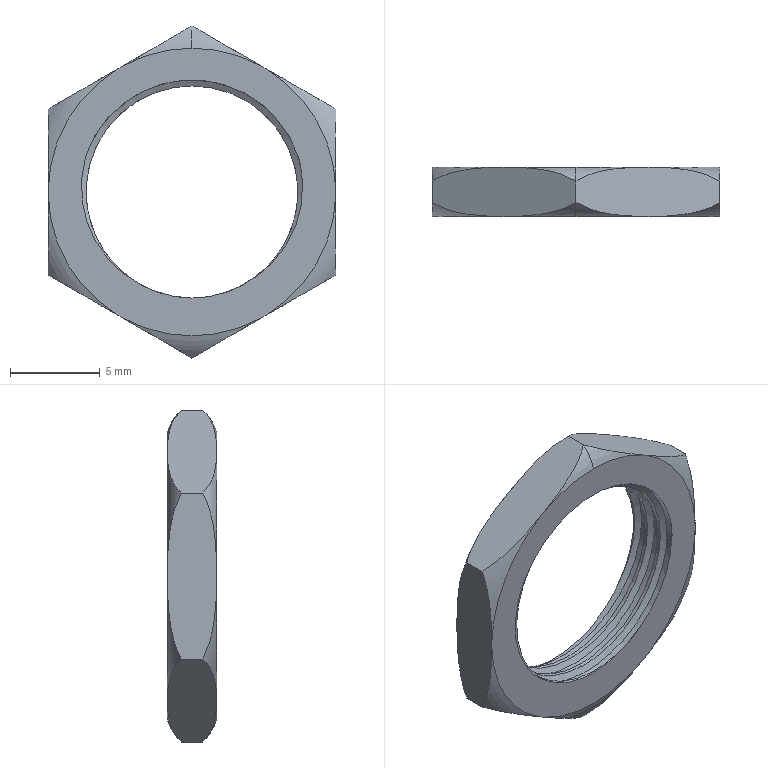Part | SolidWorks | features Extrusion 1, Helix 1, RevCut 1, SweepCut 1 | 1 solid | 32 faces | box 16 x 2.75 x 18.475 mm | volume 281.244 mm3 | torus 14 | plane 8 | cylinder 7 | spline 3 | commonest cylinder face diameters 11.8 x7